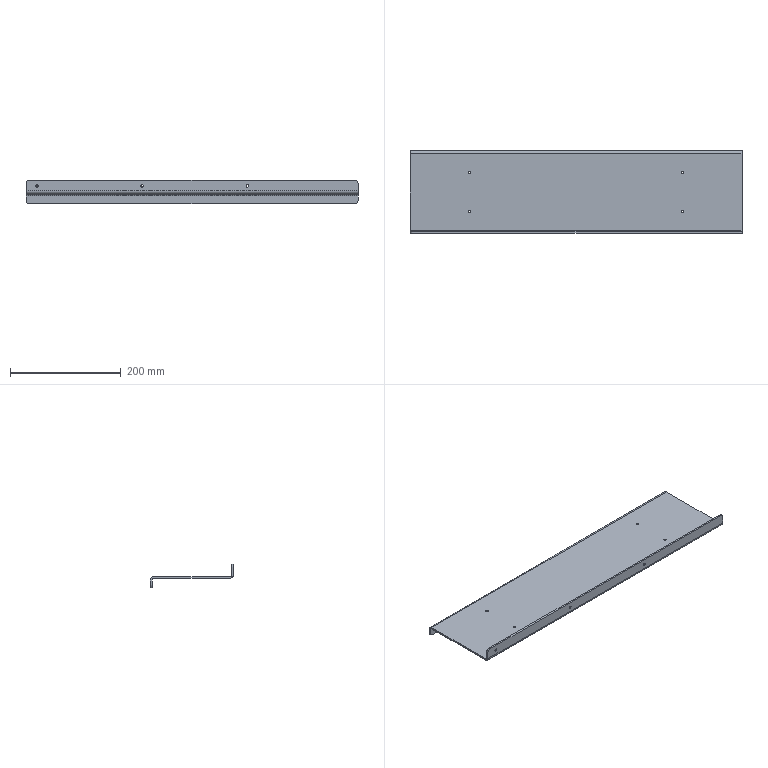Part | STEP file | J452-EBZ05-26-08-Part-1 | 1 solid | 32 faces | box 600 x 150 x 42 mm | volume 332889 mm3 | cylinder 22 | plane 10 | commonest cylinder face diameters 4 x8 4.5 x6 10 x4 6 x2 12 x2